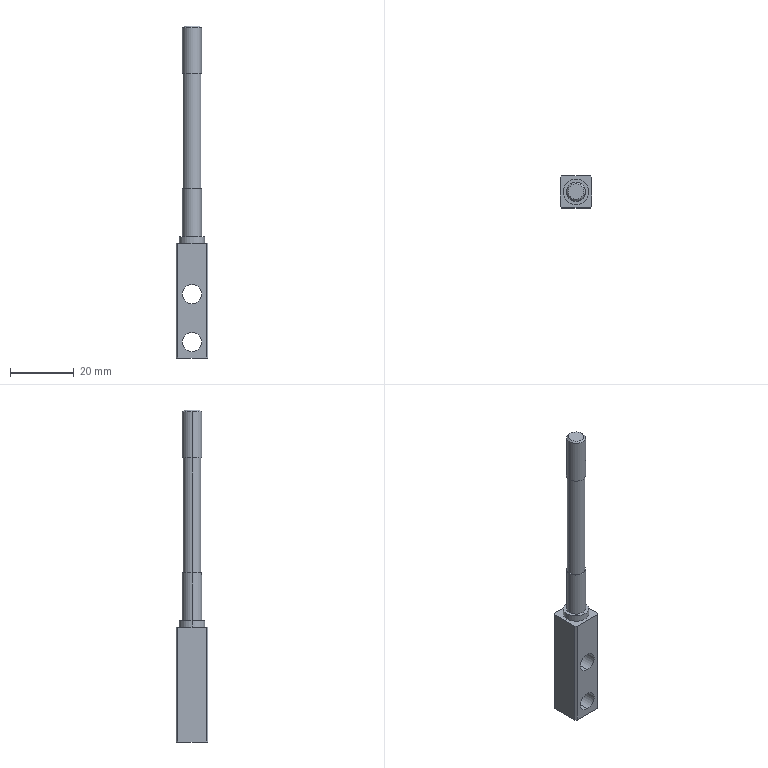Part | SolidWorks | features ICE 3, Chamfer 2, Extrusion 1, RefAxis 1, RevCut 1 | 1 solid | 28 faces | box 10 x 10 x 104 mm | volume 4818 mm3 | plane 14 | cylinder 12 | cone 2 | commonest cylinder face diameters 6 x8 5.5 x2 8 x2
STEP:
#1=CARTESIAN_POINT('',(-3.,0.,103.5));
#2=VERTEX_POINT('',#1);
#3=CARTESIAN_POINT('',(3.,0.,103.5));
#4=VERTEX_POINT('',#3);
#5=CARTESIAN_POINT('',(0.,0.,103.5));
#6=DIRECTION('',(0.,0.,-1.));
#7=DIRECTION('',(1.,0.,0.));
#8=AXIS2_PLACEMENT_3D('',#5,#6,#7);
#9=CIRCLE('',#8,3.);
#10=EDGE_CURVE('',#2,#4,#9,.T.);
#11=ORIENTED_EDGE('',*,*,#10,.T.);
#12=CARTESIAN_POINT('',(3.,0.,89.));
#13=VERTEX_POINT('',#12);
#14=CARTESIAN_POINT('',(3.,0.,104.));
#15=DIRECTION('',(0.,0.,-1.));
#16=VECTOR('',#15,1000.);
#17=LINE('',#14,#16);
#18=EDGE_CURVE('',#4,#13,#17,.T.);
#19=ORIENTED_EDGE('',*,*,#18,.T.);
#20=CARTESIAN_POINT('',(-3.,0.,89.));
#21=VERTEX_POINT('',#20);
#22=CARTESIAN_POINT('',(0.,0.,89.));
#23=DIRECTION('',(0.,0.,1.));
#24=DIRECTION('',(1.,0.,0.));
#25=AXIS2_PLACEMENT_3D('',#22,#23,#24);
#26=CIRCLE('',#25,3.);
#27=EDGE_CURVE('',#13,#21,#26,.T.);
#28=ORIENTED_EDGE('',*,*,#27,.T.);
#29=CARTESIAN_POINT('',(-3.,0.,104.));
#30=DIRECTION('',(0.,0.,-1.));
#31=VECTOR('',#30,1000.);
#32=LINE('',#29,#31);
#33=EDGE_CURVE('',#2,#21,#32,.T.);
#34=ORIENTED_EDGE('',*,*,#33,.F.);
#35=EDGE_LOOP('',(#11,#19,#28,#34));
#36=FACE_OUTER_BOUND('',#35,.T.);
#37=CARTESIAN_POINT('',(0.,0.,104.));
#38=DIRECTION('',(0.,0.,-1.));
#39=DIRECTION('',(-1.,0.,0.));
#40=AXIS2_PLACEMENT_3D('',#37,#38,#39);
#41=CYLINDRICAL_SURFACE('',#40,3.);
#42=ADVANCED_FACE('',(#36),#41,.T.);
#43=CARTESIAN_POINT('',(2.5,0.,104.));
#44=VERTEX_POINT('',#43);
#45=CARTESIAN_POINT('',(-2.5,0.,104.));
#46=VERTEX_POINT('',#45);
#47=CARTESIAN_POINT('',(0.,0.,104.));
#48=DIRECTION('',(0.,0.,1.));
#49=DIRECTION('',(1.,0.,0.));
#50=AXIS2_PLACEMENT_3D('',#47,#48,#49);
#51=CIRCLE('',#50,2.5);
#52=EDGE_CURVE('',#44,#46,#51,.T.);
#53=ORIENTED_EDGE('',*,*,#52,.F.);
#54=CARTESIAN_POINT('',(2.5,0.,104.));
#55=DIRECTION('',(0.7071,0.,-0.7071));
#56=VECTOR('',#55,1000.);
#57=LINE('',#54,#56);
#58=EDGE_CURVE('',#44,#4,#57,.T.);
#59=ORIENTED_EDGE('',*,*,#58,.T.);
#60=ORIENTED_EDGE('',*,*,#10,.F.);
#61=CARTESIAN_POINT('',(-2.5,0.,104.));
#62=DIRECTION('',(-0.7071,0.,-0.7071));
#63=VECTOR('',#62,1000.);
#64=LINE('',#61,#63);
#65=EDGE_CURVE('',#46,#2,#64,.T.);
#66=ORIENTED_EDGE('',*,*,#65,.F.);
#67=EDGE_LOOP('',(#53,#59,#60,#66));
#68=FACE_OUTER_BOUND('',#67,.T.);
#69=CARTESIAN_POINT('',(0.,0.,104.));
#70=DIRECTION('',(0.,0.,-1.));
#71=DIRECTION('',(-1.,0.,0.));
#72=AXIS2_PLACEMENT_3D('',#69,#70,#71);
#73=CONICAL_SURFACE('',#72,2.5,0.7854);
#74=ADVANCED_FACE('',(#68),#73,.T.);
#75=CARTESIAN_POINT('',(2.75,0.,53.));
#76=VERTEX_POINT('',#75);
#77=CARTESIAN_POINT('',(-2.75,0.,53.));
#78=VERTEX_POINT('',#77);
#79=CARTESIAN_POINT('',(0.,0.,53.));
#80=DIRECTION('',(0.,0.,1.));
#81=DIRECTION('',(1.,0.,0.));
#82=AXIS2_PLACEMENT_3D('',#79,#80,#81);
#83=CIRCLE('',#82,2.75);
#84=EDGE_CURVE('',#76,#78,#83,.T.);
#85=ORIENTED_EDGE('',*,*,#84,.T.);
#86=CARTESIAN_POINT('',(-2.75,0.,89.));
#87=VERTEX_POINT('',#86);
#88=CARTESIAN_POINT('',(-2.75,0.,103.5));
#89=DIRECTION('',(0.,0.,1.));
#90=VECTOR('',#89,1000.);
#91=LINE('',#88,#90);
#92=EDGE_CURVE('',#78,#87,#91,.T.);
#93=ORIENTED_EDGE('',*,*,#92,.T.);
#94=CARTESIAN_POINT('',(2.75,0.,89.));
#95=VERTEX_POINT('',#94);
#96=CARTESIAN_POINT('',(0.,0.,89.));
#97=DIRECTION('',(0.,0.,1.));
#98=DIRECTION('',(1.,0.,0.));
#99=AXIS2_PLACEMENT_3D('',#96,#97,#98);
#100=CIRCLE('',#99,2.75);
#101=EDGE_CURVE('',#95,#87,#100,.T.);
#102=ORIENTED_EDGE('',*,*,#101,.F.);
#103=CARTESIAN_POINT('',(2.75,0.,103.5));
#104=DIRECTION('',(0.,0.,1.));
#105=VECTOR('',#104,1000.);
#106=LINE('',#103,#105);
#107=EDGE_CURVE('',#76,#95,#106,.T.);
#108=ORIENTED_EDGE('',*,*,#107,.F.);
#109=EDGE_LOOP('',(#85,#93,#102,#108));
#110=FACE_OUTER_BOUND('',#109,.T.);
#111=CARTESIAN_POINT('',(0.,0.,103.5));
#112=DIRECTION('',(0.,0.,1.));
#113=DIRECTION('',(1.,0.,0.));
#114=AXIS2_PLACEMENT_3D('',#111,#112,#113);
#115=CYLINDRICAL_SURFACE('',#114,2.75);
#116=ADVANCED_FACE('',(#110),#115,.T.);
#117=CARTESIAN_POINT('',(0.,-5.,17.));
#118=VERTEX_POINT('',#117);
#119=CARTESIAN_POINT('',(0.,-5.,23.));
#120=VERTEX_POINT('',#119);
#121=CARTESIAN_POINT('',(0.,-5.,20.));
#122=DIRECTION('',(0.,1.,0.));
#123=DIRECTION('',(0.,0.,1.));
#124=AXIS2_PLACEMENT_3D('',#121,#122,#123);
#125=CIRCLE('',#124,3.);
#126=EDGE_CURVE('',#118,#120,#125,.T.);
#127=ORIENTED_EDGE('',*,*,#126,.F.);
#128=CARTESIAN_POINT('',(0.,5.,17.));
#129=VERTEX_POINT('',#128);
#130=CARTESIAN_POINT('',(0.,-45.,17.));
#131=DIRECTION('',(0.,1.,0.));
#132=VECTOR('',#131,1000.);
#133=LINE('',#130,#132);
#134=EDGE_CURVE('',#118,#129,#133,.T.);
#135=ORIENTED_EDGE('',*,*,#134,.T.);
#136=CARTESIAN_POINT('',(0.,5.,23.));
#137=VERTEX_POINT('',#136);
#138=CARTESIAN_POINT('',(0.,5.,20.));
#139=DIRECTION('',(0.,1.,0.));
#140=DIRECTION('',(0.,0.,1.));
#141=AXIS2_PLACEMENT_3D('',#138,#139,#140);
#142=CIRCLE('',#141,3.);
#143=EDGE_CURVE('',#129,#137,#142,.T.);
#144=ORIENTED_EDGE('',*,*,#143,.T.);
#145=CARTESIAN_POINT('',(0.,-45.,23.));
#146=DIRECTION('',(0.,1.,0.));
#147=VECTOR('',#146,1000.);
#148=LINE('',#145,#147);
#149=EDGE_CURVE('',#120,#137,#148,.T.);
#150=ORIENTED_EDGE('',*,*,#149,.F.);
#151=EDGE_LOOP('',(#127,#135,#144,#150));
#152=FACE_OUTER_BOUND('',#151,.T.);
#153=CARTESIAN_POINT('',(0.,-45.,20.));
#154=DIRECTION('',(0.,1.,0.));
#155=DIRECTION('',(0.,0.,1.));
#156=AXIS2_PLACEMENT_3D('',#153,#154,#155);
#157=CYLINDRICAL_SURFACE('',#156,3.);
#158=ADVANCED_FACE('',(#152),#157,.F.);
#159=CARTESIAN_POINT('',(0.,-5.,2.));
#160=VERTEX_POINT('',#159);
#161=CARTESIAN_POINT('',(0.,-5.,8.));
#162=VERTEX_POINT('',#161);
#163=CARTESIAN_POINT('',(0.,-5.,5.));
#164=DIRECTION('',(0.,1.,0.));
#165=DIRECTION('',(0.,0.,1.));
#166=AXIS2_PLACEMENT_3D('',#163,#164,#165);
#167=CIRCLE('',#166,3.);
#168=EDGE_CURVE('',#160,#162,#167,.T.);
#169=ORIENTED_EDGE('',*,*,#168,.F.);
#170=CARTESIAN_POINT('',(0.,5.,2.));
#171=VERTEX_POINT('',#170);
#172=CARTESIAN_POINT('',(0.,-45.,2.));
#173=DIRECTION('',(0.,1.,0.));
#174=VECTOR('',#173,1000.);
#175=LINE('',#172,#174);
#176=EDGE_CURVE('',#160,#171,#175,.T.);
#177=ORIENTED_EDGE('',*,*,#176,.T.);
#178=CARTESIAN_POINT('',(0.,5.,8.));
#179=VERTEX_POINT('',#178);
#180=CARTESIAN_POINT('',(0.,5.,5.));
#181=DIRECTION('',(0.,1.,0.));
#182=DIRECTION('',(0.,0.,1.));
#183=AXIS2_PLACEMENT_3D('',#180,#181,#182);
#184=CIRCLE('',#183,3.);
#185=EDGE_CURVE('',#171,#179,#184,.T.);
#186=ORIENTED_EDGE('',*,*,#185,.T.);
#187=CARTESIAN_POINT('',(0.,-45.,8.));
#188=DIRECTION('',(0.,1.,0.));
#189=VECTOR('',#188,1000.);
#190=LINE('',#187,#189);
#191=EDGE_CURVE('',#162,#179,#190,.T.);
#192=ORIENTED_EDGE('',*,*,#191,.F.);
#193=EDGE_LOOP('',(#169,#177,#186,#192));
#194=FACE_OUTER_BOUND('',#193,.T.);
#195=CARTESIAN_POINT('',(0.,-45.,5.));
#196=DIRECTION('',(0.,1.,0.));
#197=DIRECTION('',(0.,0.,1.));
#198=AXIS2_PLACEMENT_3D('',#195,#196,#197);
#199=CYLINDRICAL_SURFACE('',#198,3.);
#200=ADVANCED_FACE('',(#194),#199,.F.);
#201=CARTESIAN_POINT('',(-3.,0.,53.));
#202=VERTEX_POINT('',#201);
#203=CARTESIAN_POINT('',(3.,0.,53.));
#204=VERTEX_POINT('',#203);
#205=CARTESIAN_POINT('',(0.,0.,53.));
#206=DIRECTION('',(0.,0.,-1.));
#207=DIRECTION('',(-1.,0.,0.));
#208=AXIS2_PLACEMENT_3D('',#205,#206,#207);
#209=CIRCLE('',#208,3.);
#210=EDGE_CURVE('',#202,#204,#209,.T.);
#211=ORIENTED_EDGE('',*,*,#210,.T.);
#212=CARTESIAN_POINT('',(3.,0.,38.));
#213=VERTEX_POINT('',#212);
#214=CARTESIAN_POINT('',(3.,0.,104.));
#215=DIRECTION('',(0.,0.,-1.));
#216=VECTOR('',#215,1000.);
#217=LINE('',#214,#216);
#218=EDGE_CURVE('',#204,#213,#217,.T.);
#219=ORIENTED_EDGE('',*,*,#218,.T.);
#220=CARTESIAN_POINT('',(-3.,0.,38.));
#221=VERTEX_POINT('',#220);
#222=CARTESIAN_POINT('',(0.,0.,38.));
#223=DIRECTION('',(0.,0.,1.));
#224=DIRECTION('',(1.,0.,0.));
#225=AXIS2_PLACEMENT_3D('',#222,#223,#224);
#226=CIRCLE('',#225,3.);
#227=EDGE_CURVE('',#213,#221,#226,.T.);
#228=ORIENTED_EDGE('',*,*,#227,.T.);
#229=CARTESIAN_POINT('',(-3.,0.,104.));
#230=DIRECTION('',(0.,0.,-1.));
#231=VECTOR('',#230,1000.);
#232=LINE('',#229,#231);
#233=EDGE_CURVE('',#202,#221,#232,.T.);
#234=ORIENTED_EDGE('',*,*,#233,.F.);
#235=EDGE_LOOP('',(#211,#219,#228,#234));
#236=FACE_OUTER_BOUND('',#235,.T.);
#237=CARTESIAN_POINT('',(0.,0.,104.));
#238=DIRECTION('',(0.,0.,-1.));
#239=DIRECTION('',(-1.,0.,0.));
#240=AXIS2_PLACEMENT_3D('',#237,#238,#239);
#241=CYLINDRICAL_SURFACE('',#240,3.);
#242=ADVANCED_FACE('',(#236),#241,.T.);
#243=CARTESIAN_POINT('',(4.,0.,38.));
#244=VERTEX_POINT('',#243);
#245=CARTESIAN_POINT('',(-4.,0.,38.));
#246=VERTEX_POINT('',#245);
#247=CARTESIAN_POINT('',(0.,0.,38.));
#248=DIRECTION('',(0.,0.,1.));
#249=DIRECTION('',(1.,0.,0.));
#250=AXIS2_PLACEMENT_3D('',#247,#248,#249);
#251=CIRCLE('',#250,4.);
#252=EDGE_CURVE('',#244,#246,#251,.T.);
#253=ORIENTED_EDGE('',*,*,#252,.F.);
#254=CARTESIAN_POINT('',(4.,0.,36.));
#255=VERTEX_POINT('',#254);
#256=CARTESIAN_POINT('',(4.,0.,38.));
#257=DIRECTION('',(0.,0.,-1.));
#258=VECTOR('',#257,1000.);
#259=LINE('',#256,#258);
#260=EDGE_CURVE('',#244,#255,#259,.T.);
#261=ORIENTED_EDGE('',*,*,#260,.T.);
#262=CARTESIAN_POINT('',(-4.,0.,36.));
#263=VERTEX_POINT('',#262);
#264=CARTESIAN_POINT('',(0.,0.,36.));
#265=DIRECTION('',(0.,0.,1.));
#266=DIRECTION('',(1.,0.,0.));
#267=AXIS2_PLACEMENT_3D('',#264,#265,#266);
#268=CIRCLE('',#267,4.);
#269=EDGE_CURVE('',#255,#263,#268,.T.);
#270=ORIENTED_EDGE('',*,*,#269,.T.);
#271=CARTESIAN_POINT('',(-4.,0.,38.));
#272=DIRECTION('',(0.,0.,-1.));
#273=VECTOR('',#272,1000.);
#274=LINE('',#271,#273);
#275=EDGE_CURVE('',#246,#263,#274,.T.);
#276=ORIENTED_EDGE('',*,*,#275,.F.);
#277=EDGE_LOOP('',(#253,#261,#270,#276));
#278=FACE_OUTER_BOUND('',#277,.T.);
#279=CARTESIAN_POINT('',(0.,0.,38.));
#280=DIRECTION('',(0.,0.,-1.));
#281=DIRECTION('',(-1.,0.,0.));
#282=AXIS2_PLACEMENT_3D('',#279,#280,#281);
#283=CYLINDRICAL_SURFACE('',#282,4.);
#284=ADVANCED_FACE('',(#278),#283,.T.);
#285=CARTESIAN_POINT('',(0.,0.,38.));
#286=DIRECTION('',(0.,0.,1.));
#287=DIRECTION('',(1.,0.,0.));
#288=AXIS2_PLACEMENT_3D('',#285,#286,#287);
#289=CIRCLE('',#288,4.);
#290=EDGE_CURVE('',#246,#244,#289,.T.);
#291=ORIENTED_EDGE('',*,*,#290,.T.);
#292=ORIENTED_EDGE('',*,*,#252,.T.);
#293=EDGE_LOOP('',(#291,#292));
#294=FACE_OUTER_BOUND('',#293,.T.);
#295=CARTESIAN_POINT('',(0.,0.,38.));
#296=DIRECTION('',(0.,0.,1.));
#297=DIRECTION('',(1.,0.,0.));
#298=AXIS2_PLACEMENT_3D('',#295,#296,#297);
#299=CIRCLE('',#298,3.);
#300=EDGE_CURVE('',#221,#213,#299,.T.);
#301=ORIENTED_EDGE('',*,*,#300,.F.);
#302=ORIENTED_EDGE('',*,*,#227,.F.);
#303=EDGE_LOOP('',(#301,#302));
#304=FACE_BOUND('',#303,.T.);
#305=CARTESIAN_POINT('',(0.,0.,38.));
#306=DIRECTION('',(0.,0.,1.));
#307=DIRECTION('',(1.,0.,0.));
#308=AXIS2_PLACEMENT_3D('',#305,#306,#307);
#309=PLANE('',#308);
#310=ADVANCED_FACE('',(#294,#304),#309,.T.);
#311=CARTESIAN_POINT('',(-4.5,-5.,36.));
#312=VERTEX_POINT('',#311);
#313=CARTESIAN_POINT('',(4.5,-5.,36.));
#314=VERTEX_POINT('',#313);
#315=CARTESIAN_POINT('',(-5.,-5.,36.));
#316=DIRECTION('',(1.,0.,0.));
#317=VECTOR('',#316,1000.);
#318=LINE('',#315,#317);
#319=EDGE_CURVE('',#312,#314,#318,.T.);
#320=ORIENTED_EDGE('',*,*,#319,.T.);
#321=CARTESIAN_POINT('',(5.,-4.5,36.));
#322=VERTEX_POINT('',#321);
#323=CARTESIAN_POINT('',(4.75,-4.75,36.));
#324=DIRECTION('',(0.7071,0.7071,0.));
#325=VECTOR('',#324,1000.);
#326=LINE('',#323,#325);
#327=EDGE_CURVE('',#314,#322,#326,.T.);
#328=ORIENTED_EDGE('',*,*,#327,.T.);
#329=CARTESIAN_POINT('',(5.,4.5,36.));
#330=VERTEX_POINT('',#329);
#331=CARTESIAN_POINT('',(5.,5.,36.));
#332=DIRECTION('',(0.,1.,0.));
#333=VECTOR('',#332,1000.);
#334=LINE('',#331,#333);
#335=EDGE_CURVE('',#322,#330,#334,.T.);
#336=ORIENTED_EDGE('',*,*,#335,.T.);
#337=CARTESIAN_POINT('',(4.5,5.,36.));
#338=VERTEX_POINT('',#337);
#339=CARTESIAN_POINT('',(9.75,-0.25,36.));
#340=DIRECTION('',(-0.7071,0.7071,0.));
#341=VECTOR('',#340,1000.);
#342=LINE('',#339,#341);
#343=EDGE_CURVE('',#330,#338,#342,.T.);
#344=ORIENTED_EDGE('',*,*,#343,.T.);
#345=CARTESIAN_POINT('',(-4.5,5.,36.));
#346=VERTEX_POINT('',#345);
#347=CARTESIAN_POINT('',(-5.,5.,36.));
#348=DIRECTION('',(-1.,0.,0.));
#349=VECTOR('',#348,1000.);
#350=LINE('',#347,#349);
#351=EDGE_CURVE('',#338,#346,#350,.T.);
#352=ORIENTED_EDGE('',*,*,#351,.T.);
#353=CARTESIAN_POINT('',(-5.,4.5,36.));
#354=VERTEX_POINT('',#353);
#355=CARTESIAN_POINT('',(-4.75,4.75,36.));
#356=DIRECTION('',(-0.7071,-0.7071,0.));
#357=VECTOR('',#356,1000.);
#358=LINE('',#355,#357);
#359=EDGE_CURVE('',#346,#354,#358,.T.);
#360=ORIENTED_EDGE('',*,*,#359,.T.);
#361=CARTESIAN_POINT('',(-5.,-4.5,36.));
#362=VERTEX_POINT('',#361);
#363=CARTESIAN_POINT('',(-5.,5.,36.));
#364=DIRECTION('',(0.,-1.,0.));
#365=VECTOR('',#364,1000.);
#366=LINE('',#363,#365);
#367=EDGE_CURVE('',#354,#362,#366,.T.);
#368=ORIENTED_EDGE('',*,*,#367,.T.);
#369=CARTESIAN_POINT('',(0.25,-9.75,36.));
#370=DIRECTION('',(0.7071,-0.7071,0.));
#371=VECTOR('',#370,1000.);
#372=LINE('',#369,#371);
#373=EDGE_CURVE('',#362,#312,#372,.T.);
#374=ORIENTED_EDGE('',*,*,#373,.T.);
#375=EDGE_LOOP('',(#320,#328,#336,#344,#352,#360,#368,#374));
#376=FACE_OUTER_BOUND('',#375,.T.);
#377=CARTESIAN_POINT('',(0.,0.,36.));
#378=DIRECTION('',(0.,0.,1.));
#379=DIRECTION('',(1.,0.,0.));
#380=AXIS2_PLACEMENT_3D('',#377,#378,#379);
#381=CIRCLE('',#380,4.);
#382=EDGE_CURVE('',#263,#255,#381,.T.);
#383=ORIENTED_EDGE('',*,*,#382,.F.);
#384=ORIENTED_EDGE('',*,*,#269,.F.);
#385=EDGE_LOOP('',(#383,#384));
#386=FACE_BOUND('',#385,.T.);
#387=CARTESIAN_POINT('',(5.,-5.,36.));
#388=DIRECTION('',(0.,0.,1.));
#389=DIRECTION('',(1.,0.,0.));
#390=AXIS2_PLACEMENT_3D('',#387,#388,#389);
#391=PLANE('',#390);
#392=ADVANCED_FACE('',(#376,#386),#391,.T.);
#393=ORIENTED_EDGE('',*,*,#335,.F.);
#394=CARTESIAN_POINT('',(5.,-4.5,0.));
#395=VERTEX_POINT('',#394);
#396=CARTESIAN_POINT('',(5.,-4.5,36.));
#397=DIRECTION('',(0.,0.,-1.));
#398=VECTOR('',#397,1000.);
#399=LINE('',#396,#398);
#400=EDGE_CURVE('',#322,#395,#399,.T.);
#401=ORIENTED_EDGE('',*,*,#400,.T.);
#402=CARTESIAN_POINT('',(5.,4.5,0.));
#403=VERTEX_POINT('',#402);
#404=CARTESIAN_POINT('',(5.,5.,0.));
#405=DIRECTION('',(0.,1.,0.));
#406=VECTOR('',#405,1000.);
#407=LINE('',#404,#406);
#408=EDGE_CURVE('',#395,#403,#407,.T.);
#409=ORIENTED_EDGE('',*,*,#408,.T.);
#410=CARTESIAN_POINT('',(5.,4.5,36.));
#411=DIRECTION('',(0.,0.,1.));
#412=VECTOR('',#411,1000.);
#413=LINE('',#410,#412);
#414=EDGE_CURVE('',#403,#330,#413,.T.);
#415=ORIENTED_EDGE('',*,*,#414,.T.);
#416=EDGE_LOOP('',(#393,#401,#409,#415));
#417=FACE_OUTER_BOUND('',#416,.T.);
#418=CARTESIAN_POINT('',(5.,5.,36.));
#419=DIRECTION('',(-1.,0.,0.));
#420=DIRECTION('',(0.,0.,1.));
#421=AXIS2_PLACEMENT_3D('',#418,#419,#420);
#422=PLANE('',#421);
#423=ADVANCED_FACE('',(#417),#422,.F.);
#424=CARTESIAN_POINT('',(0.,5.,20.));
#425=DIRECTION('',(0.,1.,0.));
#426=DIRECTION('',(0.,0.,1.));
#427=AXIS2_PLACEMENT_3D('',#424,#425,#426);
#428=CIRCLE('',#427,3.);
#429=EDGE_CURVE('',#137,#129,#428,.T.);
#430=ORIENTED_EDGE('',*,*,#429,.F.);
#431=ORIENTED_EDGE('',*,*,#143,.F.);
#432=EDGE_LOOP('',(#430,#431));
#433=FACE_BOUND('',#432,.T.);
#434=CARTESIAN_POINT('',(0.,5.,5.));
#435=DIRECTION('',(0.,1.,0.));
#436=DIRECTION('',(0.,0.,1.));
#437=AXIS2_PLACEMENT_3D('',#434,#435,#436);
#438=CIRCLE('',#437,3.);
#439=EDGE_CURVE('',#179,#171,#438,.T.);
#440=ORIENTED_EDGE('',*,*,#439,.F.);
#441=ORIENTED_EDGE('',*,*,#185,.F.);
#442=EDGE_LOOP('',(#440,#441));
#443=FACE_BOUND('',#442,.T.);
#444=ORIENTED_EDGE('',*,*,#351,.F.);
#445=CARTESIAN_POINT('',(4.5,5.,0.));
#446=VERTEX_POINT('',#445);
#447=CARTESIAN_POINT('',(4.5,5.,36.));
#448=DIRECTION('',(0.,0.,-1.));
#449=VECTOR('',#448,1000.);
#450=LINE('',#447,#449);
#451=EDGE_CURVE('',#338,#446,#450,.T.);
#452=ORIENTED_EDGE('',*,*,#451,.T.);
#453=CARTESIAN_POINT('',(-4.5,5.,0.));
#454=VERTEX_POINT('',#453);
#455=CARTESIAN_POINT('',(-5.,5.,0.));
#456=DIRECTION('',(-1.,0.,0.));
#457=VECTOR('',#456,1000.);
#458=LINE('',#455,#457);
#459=EDGE_CURVE('',#446,#454,#458,.T.);
#460=ORIENTED_EDGE('',*,*,#459,.T.);
#461=CARTESIAN_POINT('',(-4.5,5.,36.));
#462=DIRECTION('',(0.,0.,1.));
#463=VECTOR('',#462,1000.);
#464=LINE('',#461,#463);
#465=EDGE_CURVE('',#454,#346,#464,.T.);
#466=ORIENTED_EDGE('',*,*,#465,.T.);
#467=EDGE_LOOP('',(#444,#452,#460,#466));
#468=FACE_OUTER_BOUND('',#467,.T.);
#469=CARTESIAN_POINT('',(-5.,5.,36.));
#470=DIRECTION('',(0.,-1.,0.));
#471=DIRECTION('',(0.,0.,-1.));
#472=AXIS2_PLACEMENT_3D('',#469,#470,#471);
#473=PLANE('',#472);
#474=ADVANCED_FACE('',(#433,#443,#468),#473,.F.);
#475=ORIENTED_EDGE('',*,*,#367,.F.);
#476=CARTESIAN_POINT('',(-5.,4.5,0.));
#477=VERTEX_POINT('',#476);
#478=CARTESIAN_POINT('',(-5.,4.5,36.));
#479=DIRECTION('',(0.,0.,-1.));
#480=VECTOR('',#479,1000.);
#481=LINE('',#478,#480);
#482=EDGE_CURVE('',#354,#477,#481,.T.);
#483=ORIENTED_EDGE('',*,*,#482,.T.);
#484=CARTESIAN_POINT('',(-5.,-4.5,0.));
#485=VERTEX_POINT('',#484);
#486=CARTESIAN_POINT('',(-5.,5.,0.));
#487=DIRECTION('',(0.,-1.,0.));
#488=VECTOR('',#487,1000.);
#489=LINE('',#486,#488);
#490=EDGE_CURVE('',#477,#485,#489,.T.);
#491=ORIENTED_EDGE('',*,*,#490,.T.);
#492=CARTESIAN_POINT('',(-5.,-4.5,36.));
#493=DIRECTION('',(0.,0.,1.));
#494=VECTOR('',#493,1000.);
#495=LINE('',#492,#494);
#496=EDGE_CURVE('',#485,#362,#495,.T.);
#497=ORIENTED_EDGE('',*,*,#496,.T.);
#498=EDGE_LOOP('',(#475,#483,#491,#497));
#499=FACE_OUTER_BOUND('',#498,.T.);
#500=CARTESIAN_POINT('',(-5.,5.,36.));
#501=DIRECTION('',(1.,0.,0.));
#502=DIRECTION('',(0.,1.,0.));
#503=AXIS2_PLACEMENT_3D('',#500,#501,#502);
#504=PLANE('',#503);
#505=ADVANCED_FACE('',(#499),#504,.F.);
#506=CARTESIAN_POINT('',(0.,-5.,20.));
#507=DIRECTION('',(0.,1.,0.));
#508=DIRECTION('',(0.,0.,1.));
#509=AXIS2_PLACEMENT_3D('',#506,#507,#508);
#510=CIRCLE('',#509,3.);
#511=EDGE_CURVE('',#120,#118,#510,.T.);
#512=ORIENTED_EDGE('',*,*,#511,.T.);
#513=ORIENTED_EDGE('',*,*,#126,.T.);
#514=EDGE_LOOP('',(#512,#513));
#515=FACE_BOUND('',#514,.T.);
#516=CARTESIAN_POINT('',(0.,-5.,5.));
#517=DIRECTION('',(0.,1.,0.));
#518=DIRECTION('',(0.,0.,1.));
#519=AXIS2_PLACEMENT_3D('',#516,#517,#518);
#520=CIRCLE('',#519,3.);
#521=EDGE_CURVE('',#162,#160,#520,.T.);
#522=ORIENTED_EDGE('',*,*,#521,.T.);
#523=ORIENTED_EDGE('',*,*,#168,.T.);
#524=EDGE_LOOP('',(#522,#523));
#525=FACE_BOUND('',#524,.T.);
#526=CARTESIAN_POINT('',(-4.5,-5.,0.));
#527=VERTEX_POINT('',#526);
#528=CARTESIAN_POINT('',(4.5,-5.,0.));
#529=VERTEX_POINT('',#528);
#530=CARTESIAN_POINT('',(-5.,-5.,0.));
#531=DIRECTION('',(1.,0.,0.));
#532=VECTOR('',#531,1000.);
#533=LINE('',#530,#532);
#534=EDGE_CURVE('',#527,#529,#533,.T.);
#535=ORIENTED_EDGE('',*,*,#534,.T.);
#536=CARTESIAN_POINT('',(4.5,-5.,36.));
#537=DIRECTION('',(0.,0.,1.));
#538=VECTOR('',#537,1000.);
#539=LINE('',#536,#538);
#540=EDGE_CURVE('',#529,#314,#539,.T.);
#541=ORIENTED_EDGE('',*,*,#540,.T.);
#542=ORIENTED_EDGE('',*,*,#319,.F.);
#543=CARTESIAN_POINT('',(-4.5,-5.,36.));
#544=DIRECTION('',(0.,0.,-1.));
#545=VECTOR('',#544,1000.);
#546=LINE('',#543,#545);
#547=EDGE_CURVE('',#312,#527,#546,.T.);
#548=ORIENTED_EDGE('',*,*,#547,.T.);
#549=EDGE_LOOP('',(#535,#541,#542,#548));
#550=FACE_OUTER_BOUND('',#549,.T.);
#551=CARTESIAN_POINT('',(-5.,-5.,36.));
#552=DIRECTION('',(0.,1.,0.));
#553=DIRECTION('',(0.,0.,1.));
#554=AXIS2_PLACEMENT_3D('',#551,#552,#553);
#555=PLANE('',#554);
#556=ADVANCED_FACE('',(#515,#525,#550),#555,.F.);
#557=ORIENTED_EDGE('',*,*,#408,.F.);
#558=CARTESIAN_POINT('',(5.,-4.5,0.));
#559=DIRECTION('',(-0.7071,-0.7071,0.));
#560=VECTOR('',#559,1000.);
#561=LINE('',#558,#560);
#562=EDGE_CURVE('',#395,#529,#561,.T.);
#563=ORIENTED_EDGE('',*,*,#562,.T.);
#564=ORIENTED_EDGE('',*,*,#534,.F.);
#565=CARTESIAN_POINT('',(-4.5,-5.,0.));
#566=DIRECTION('',(-0.7071,0.7071,0.));
#567=VECTOR('',#566,1000.);
#568=LINE('',#565,#567);
#569=EDGE_CURVE('',#527,#485,#568,.T.);
#570=ORIENTED_EDGE('',*,*,#569,.T.);
#571=ORIENTED_EDGE('',*,*,#490,.F.);
#572=CARTESIAN_POINT('',(-5.,4.5,0.));
#573=DIRECTION('',(0.7071,0.7071,0.));
#574=VECTOR('',#573,1000.);
#575=LINE('',#572,#574);
#576=EDGE_CURVE('',#477,#454,#575,.T.);
#577=ORIENTED_EDGE('',*,*,#576,.T.);
#578=ORIENTED_EDGE('',*,*,#459,.F.);
#579=CARTESIAN_POINT('',(4.5,5.,0.));
#580=DIRECTION('',(0.7071,-0.7071,0.));
#581=VECTOR('',#580,1000.);
#582=LINE('',#579,#581);
#583=EDGE_CURVE('',#446,#403,#582,.T.);
#584=ORIENTED_EDGE('',*,*,#583,.T.);
#585=EDGE_LOOP('',(#557,#563,#564,#570,#571,#577,#578,#584));
#586=FACE_OUTER_BOUND('',#585,.T.);
#587=CARTESIAN_POINT('',(5.,-5.,0.));
#588=DIRECTION('',(0.,0.,1.));
#589=DIRECTION('',(1.,0.,0.));
#590=AXIS2_PLACEMENT_3D('',#587,#588,#589);
#591=PLANE('',#590);
#592=ADVANCED_FACE('',(#586),#591,.F.);
#593=ORIENTED_EDGE('',*,*,#260,.F.);
#594=ORIENTED_EDGE('',*,*,#290,.F.);
#595=ORIENTED_EDGE('',*,*,#275,.T.);
#596=ORIENTED_EDGE('',*,*,#382,.T.);
#597=EDGE_LOOP('',(#593,#594,#595,#596));
#598=FACE_OUTER_BOUND('',#597,.T.);
#599=CARTESIAN_POINT('',(0.,0.,38.));
#600=DIRECTION('',(0.,0.,-1.));
#601=DIRECTION('',(-1.,0.,0.));
#602=AXIS2_PLACEMENT_3D('',#599,#600,#601);
#603=CYLINDRICAL_SURFACE('',#602,4.);
#604=ADVANCED_FACE('',(#598),#603,.T.);
#605=ORIENTED_EDGE('',*,*,#218,.F.);
#606=CARTESIAN_POINT('',(0.,0.,53.));
#607=DIRECTION('',(0.,0.,-1.));
#608=DIRECTION('',(-1.,0.,0.));
#609=AXIS2_PLACEMENT_3D('',#606,#607,#608);
#610=CIRCLE('',#609,3.);
#611=EDGE_CURVE('',#204,#202,#610,.T.);
#612=ORIENTED_EDGE('',*,*,#611,.T.);
#613=ORIENTED_EDGE('',*,*,#233,.T.);
#614=ORIENTED_EDGE('',*,*,#300,.T.);
#615=EDGE_LOOP('',(#605,#612,#613,#614));
#616=FACE_OUTER_BOUND('',#615,.T.);
#617=CARTESIAN_POINT('',(0.,0.,104.));
#618=DIRECTION('',(0.,0.,-1.));
#619=DIRECTION('',(-1.,0.,0.));
#620=AXIS2_PLACEMENT_3D('',#617,#618,#619);
#621=CYLINDRICAL_SURFACE('',#620,3.);
#622=ADVANCED_FACE('',(#616),#621,.T.);
#623=ORIENTED_EDGE('',*,*,#176,.F.);
#624=ORIENTED_EDGE('',*,*,#521,.F.);
#625=ORIENTED_EDGE('',*,*,#191,.T.);
#626=ORIENTED_EDGE('',*,*,#439,.T.);
#627=EDGE_LOOP('',(#623,#624,#625,#626));
#628=FACE_OUTER_BOUND('',#627,.T.);
#629=CARTESIAN_POINT('',(0.,-45.,5.));
#630=DIRECTION('',(0.,1.,0.));
#631=DIRECTION('',(0.,0.,1.));
#632=AXIS2_PLACEMENT_3D('',#629,#630,#631);
#633=CYLINDRICAL_SURFACE('',#632,3.);
#634=ADVANCED_FACE('',(#628),#633,.F.);
#635=ORIENTED_EDGE('',*,*,#134,.F.);
#636=ORIENTED_EDGE('',*,*,#511,.F.);
#637=ORIENTED_EDGE('',*,*,#149,.T.);
#638=ORIENTED_EDGE('',*,*,#429,.T.);
#639=EDGE_LOOP('',(#635,#636,#637,#638));
#640=FACE_OUTER_BOUND('',#639,.T.);
#641=CARTESIAN_POINT('',(0.,-45.,20.));
#642=DIRECTION('',(0.,1.,0.));
#643=DIRECTION('',(0.,0.,1.));
#644=AXIS2_PLACEMENT_3D('',#641,#642,#643);
#645=CYLINDRICAL_SURFACE('',#644,3.);
#646=ADVANCED_FACE('',(#640),#645,.F.);
#647=ORIENTED_EDGE('',*,*,#327,.F.);
#648=ORIENTED_EDGE('',*,*,#540,.F.);
#649=ORIENTED_EDGE('',*,*,#562,.F.);
#650=ORIENTED_EDGE('',*,*,#400,.F.);
#651=EDGE_LOOP('',(#647,#648,#649,#650));
#652=FACE_OUTER_BOUND('',#651,.T.);
#653=CARTESIAN_POINT('',(5.,-4.5,36.));
#654=DIRECTION('',(-0.7071,0.7071,0.));
#655=DIRECTION('',(-0.7071,-0.7071,0.));
#656=AXIS2_PLACEMENT_3D('',#653,#654,#655);
#657=PLANE('',#656);
#658=ADVANCED_FACE('',(#652),#657,.F.);
#659=ORIENTED_EDGE('',*,*,#343,.F.);
#660=ORIENTED_EDGE('',*,*,#414,.F.);
#661=ORIENTED_EDGE('',*,*,#583,.F.);
#662=ORIENTED_EDGE('',*,*,#451,.F.);
#663=EDGE_LOOP('',(#659,#660,#661,#662));
#664=FACE_OUTER_BOUND('',#663,.T.);
#665=CARTESIAN_POINT('',(4.5,5.,36.));
#666=DIRECTION('',(-0.7071,-0.7071,0.));
#667=DIRECTION('',(0.7071,-0.7071,0.));
#668=AXIS2_PLACEMENT_3D('',#665,#666,#667);
#669=PLANE('',#668);
#670=ADVANCED_FACE('',(#664),#669,.F.);
#671=ORIENTED_EDGE('',*,*,#359,.F.);
#672=ORIENTED_EDGE('',*,*,#465,.F.);
#673=ORIENTED_EDGE('',*,*,#576,.F.);
#674=ORIENTED_EDGE('',*,*,#482,.F.);
#675=EDGE_LOOP('',(#671,#672,#673,#674));
#676=FACE_OUTER_BOUND('',#675,.T.);
#677=CARTESIAN_POINT('',(-5.,4.5,36.));
#678=DIRECTION('',(0.7071,-0.7071,0.));
#679=DIRECTION('',(0.7071,0.7071,0.));
#680=AXIS2_PLACEMENT_3D('',#677,#678,#679);
#681=PLANE('',#680);
#682=ADVANCED_FACE('',(#676),#681,.F.);
#683=ORIENTED_EDGE('',*,*,#373,.F.);
#684=ORIENTED_EDGE('',*,*,#496,.F.);
#685=ORIENTED_EDGE('',*,*,#569,.F.);
#686=ORIENTED_EDGE('',*,*,#547,.F.);
#687=EDGE_LOOP('',(#683,#684,#685,#686));
#688=FACE_OUTER_BOUND('',#687,.T.);
#689=CARTESIAN_POINT('',(-4.5,-5.,36.));
#690=DIRECTION('',(0.7071,0.7071,0.));
#691=DIRECTION('',(-0.7071,0.7071,0.));
#692=AXIS2_PLACEMENT_3D('',#689,#690,#691);
#693=PLANE('',#692);
#694=ADVANCED_FACE('',(#688),#693,.F.);
#695=ORIENTED_EDGE('',*,*,#101,.T.);
#696=CARTESIAN_POINT('',(0.,0.,89.));
#697=DIRECTION('',(0.,0.,1.));
#698=DIRECTION('',(1.,0.,0.));
#699=AXIS2_PLACEMENT_3D('',#696,#697,#698);
#700=CIRCLE('',#699,2.75);
#701=EDGE_CURVE('',#87,#95,#700,.T.);
#702=ORIENTED_EDGE('',*,*,#701,.T.);
#703=EDGE_LOOP('',(#695,#702));
#704=FACE_BOUND('',#703,.T.);
#705=CARTESIAN_POINT('',(0.,0.,89.));
#706=DIRECTION('',(0.,0.,1.));
#707=DIRECTION('',(1.,0.,0.));
#708=AXIS2_PLACEMENT_3D('',#705,#706,#707);
#709=CIRCLE('',#708,3.);
#710=EDGE_CURVE('',#21,#13,#709,.T.);
#711=ORIENTED_EDGE('',*,*,#710,.F.);
#712=ORIENTED_EDGE('',*,*,#27,.F.);
#713=EDGE_LOOP('',(#711,#712));
#714=FACE_OUTER_BOUND('',#713,.T.);
#715=CARTESIAN_POINT('',(2.75,0.,89.));
#716=DIRECTION('',(0.,0.,1.));
#717=DIRECTION('',(1.,0.,0.));
#718=AXIS2_PLACEMENT_3D('',#715,#716,#717);
#719=PLANE('',#718);
#720=ADVANCED_FACE('',(#704,#714),#719,.F.);
#721=ORIENTED_EDGE('',*,*,#84,.F.);
#722=CARTESIAN_POINT('',(0.,0.,53.));
#723=DIRECTION('',(0.,0.,1.));
#724=DIRECTION('',(1.,0.,0.));
#725=AXIS2_PLACEMENT_3D('',#722,#723,#724);
#726=CIRCLE('',#725,2.75);
#727=EDGE_CURVE('',#78,#76,#726,.T.);
#728=ORIENTED_EDGE('',*,*,#727,.F.);
#729=EDGE_LOOP('',(#721,#728));
#730=FACE_BOUND('',#729,.T.);
#731=ORIENTED_EDGE('',*,*,#210,.F.);
#732=ORIENTED_EDGE('',*,*,#611,.F.);
#733=EDGE_LOOP('',(#731,#732));
#734=FACE_OUTER_BOUND('',#733,.T.);
#735=CARTESIAN_POINT('',(2.75,0.,53.));
#736=DIRECTION('',(0.,0.,-1.));
#737=DIRECTION('',(-1.,0.,0.));
#738=AXIS2_PLACEMENT_3D('',#735,#736,#737);
#739=PLANE('',#738);
#740=ADVANCED_FACE('',(#730,#734),#739,.F.);
#741=ORIENTED_EDGE('',*,*,#92,.F.);
#742=ORIENTED_EDGE('',*,*,#727,.T.);
#743=ORIENTED_EDGE('',*,*,#107,.T.);
#744=ORIENTED_EDGE('',*,*,#701,.F.);
#745=EDGE_LOOP('',(#741,#742,#743,#744));
#746=FACE_OUTER_BOUND('',#745,.T.);
#747=CARTESIAN_POINT('',(0.,0.,103.5));
#748=DIRECTION('',(0.,0.,1.));
#749=DIRECTION('',(1.,0.,0.));
#750=AXIS2_PLACEMENT_3D('',#747,#748,#749);
#751=CYLINDRICAL_SURFACE('',#750,2.75);
#752=ADVANCED_FACE('',(#746),#751,.T.);
#753=CARTESIAN_POINT('',(0.,0.,104.));
#754=DIRECTION('',(0.,0.,1.));
#755=DIRECTION('',(1.,0.,0.));
#756=AXIS2_PLACEMENT_3D('',#753,#754,#755);
#757=CIRCLE('',#756,2.5);
#758=EDGE_CURVE('',#46,#44,#757,.T.);
#759=ORIENTED_EDGE('',*,*,#758,.T.);
#760=ORIENTED_EDGE('',*,*,#52,.T.);
#761=EDGE_LOOP('',(#759,#760));
#762=FACE_OUTER_BOUND('',#761,.T.);
#763=CARTESIAN_POINT('',(0.,0.,104.));
#764=DIRECTION('',(0.,0.,1.));
#765=DIRECTION('',(1.,0.,0.));
#766=AXIS2_PLACEMENT_3D('',#763,#764,#765);
#767=PLANE('',#766);
#768=ADVANCED_FACE('',(#762),#767,.T.);
#769=ORIENTED_EDGE('',*,*,#58,.F.);
#770=ORIENTED_EDGE('',*,*,#758,.F.);
#771=ORIENTED_EDGE('',*,*,#65,.T.);
#772=CARTESIAN_POINT('',(0.,0.,103.5));
#773=DIRECTION('',(0.,0.,-1.));
#774=DIRECTION('',(1.,0.,0.));
#775=AXIS2_PLACEMENT_3D('',#772,#773,#774);
#776=CIRCLE('',#775,3.);
#777=EDGE_CURVE('',#4,#2,#776,.T.);
#778=ORIENTED_EDGE('',*,*,#777,.F.);
#779=EDGE_LOOP('',(#769,#770,#771,#778));
#780=FACE_OUTER_BOUND('',#779,.T.);
#781=CARTESIAN_POINT('',(0.,0.,104.));
#782=DIRECTION('',(0.,0.,-1.));
#783=DIRECTION('',(-1.,0.,0.));
#784=AXIS2_PLACEMENT_3D('',#781,#782,#783);
#785=CONICAL_SURFACE('',#784,2.5,0.7854);
#786=ADVANCED_FACE('',(#780),#785,.T.);
#787=ORIENTED_EDGE('',*,*,#18,.F.);
#788=ORIENTED_EDGE('',*,*,#777,.T.);
#789=ORIENTED_EDGE('',*,*,#33,.T.);
#790=ORIENTED_EDGE('',*,*,#710,.T.);
#791=EDGE_LOOP('',(#787,#788,#789,#790));
#792=FACE_OUTER_BOUND('',#791,.T.);
#793=CARTESIAN_POINT('',(0.,0.,104.));
#794=DIRECTION('',(0.,0.,-1.));
#795=DIRECTION('',(-1.,0.,0.));
#796=AXIS2_PLACEMENT_3D('',#793,#794,#795);
#797=CYLINDRICAL_SURFACE('',#796,3.);
#798=ADVANCED_FACE('',(#792),#797,.T.);
#799=CLOSED_SHELL('',(#42,#74,#116,#158,#200,#242,#284,#310,#392,#423,#474,#505,#556,#592,#604,#622,#634,#646,#658,#670,#682,#694,#720,#740,#752,#768,#786,#798));
#800=MANIFOLD_SOLID_BREP('',#799);
#801=CARTESIAN_POINT('',(0.,0.,0.));
#802=DIRECTION('',(0.,0.,1.));
#803=DIRECTION('',(1.,0.,0.));
#804=AXIS2_PLACEMENT_3D('',#801,#802,#803);
#805=(LENGTH_UNIT()NAMED_UNIT(*)SI_UNIT(.MILLI.,.METRE.));
#806=UNCERTAINTY_MEASURE_WITH_UNIT(LENGTH_MEASURE(0.00001),#805,'','');
#807=(NAMED_UNIT(*)PLANE_ANGLE_UNIT()SI_UNIT($,.RADIAN.));
#808=(NAMED_UNIT(*)SI_UNIT($,.STERADIAN.)SOLID_ANGLE_UNIT());
#809=(GEOMETRIC_REPRESENTATION_CONTEXT(3)GLOBAL_UNCERTAINTY_ASSIGNED_CONTEXT((#806))GLOBAL_UNIT_ASSIGNED_CONTEXT((#805,#807,#808))REPRESENTATION_CONTEXT('',''));
#810=ADVANCED_BREP_SHAPE_REPRESENTATION('',(#800,#804),#809);